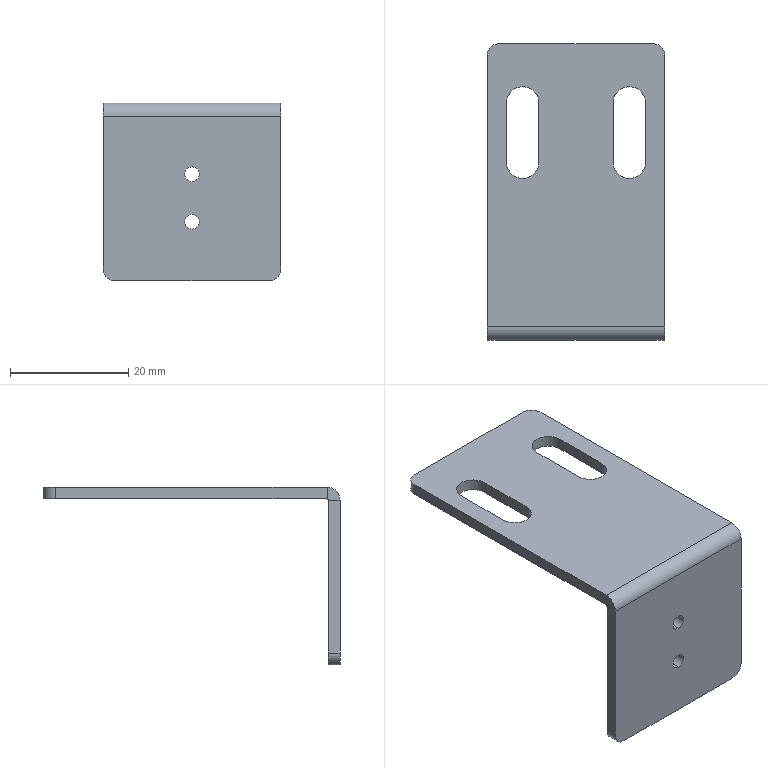Part | STEP file | Cable carrier support plate C | 1 solid | 30 faces | box 30 x 50 x 30 mm | volume 4308 mm3 | plane 16 | cylinder 14 | commonest cylinder face diameters 2.5 x4 4 x4 5.5 x4 0.4 x1 4.4 x1